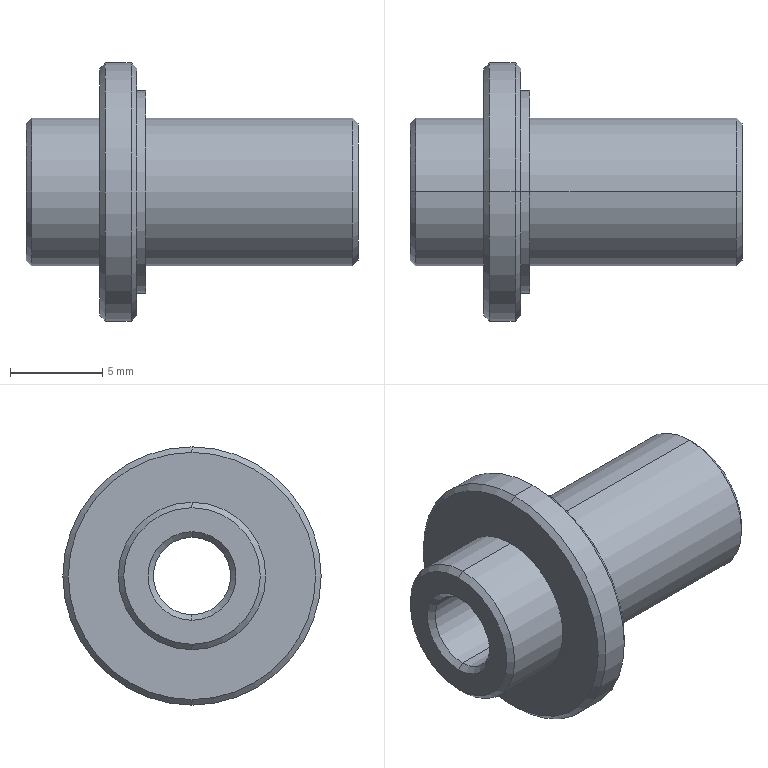Part | NX | features BREP 1 | 1 solid | 27 faces | box 18 x 14 x 14 mm | volume 877.777 mm3 | cone 12 | cylinder 10 | plane 5 | commonest cylinder face diameters 8 x4 4.2 x2 11 x2 14 x2
STEP:
#1=CARTESIAN_POINT('',(17.7,0.,2.1));
#2=VERTEX_POINT('',#1);
#3=CARTESIAN_POINT('',(17.7,0.,-2.1));
#4=VERTEX_POINT('',#3);
#5=CARTESIAN_POINT('',(17.7,0.,0.));
#6=DIRECTION('',(1.,0.,0.));
#7=DIRECTION('',(0.,0.,-1.));
#8=AXIS2_PLACEMENT_3D('',#5,#6,#7);
#9=CIRCLE('',#8,2.1);
#10=EDGE_CURVE('',#2,#4,#9,.T.);
#11=ORIENTED_EDGE('',*,*,#10,.F.);
#12=CARTESIAN_POINT('',(18.,0.,2.4));
#13=VERTEX_POINT('',#12);
#14=CARTESIAN_POINT('',(18.,0.,2.4));
#15=DIRECTION('',(0.7071,0.,0.7071));
#16=VECTOR('',#15,1000.);
#17=LINE('',#14,#16);
#18=EDGE_CURVE('',#2,#13,#17,.T.);
#19=ORIENTED_EDGE('',*,*,#18,.T.);
#20=CARTESIAN_POINT('',(18.,0.,-2.4));
#21=VERTEX_POINT('',#20);
#22=CARTESIAN_POINT('',(18.,0.,0.));
#23=DIRECTION('',(-1.,0.,0.));
#24=DIRECTION('',(0.,0.,-1.));
#25=AXIS2_PLACEMENT_3D('',#22,#23,#24);
#26=CIRCLE('',#25,2.4);
#27=EDGE_CURVE('',#21,#13,#26,.T.);
#28=ORIENTED_EDGE('',*,*,#27,.F.);
#29=CARTESIAN_POINT('',(18.,0.,-2.4));
#30=DIRECTION('',(0.7071,0.,-0.7071));
#31=VECTOR('',#30,1000.);
#32=LINE('',#29,#31);
#33=EDGE_CURVE('',#4,#21,#32,.T.);
#34=ORIENTED_EDGE('',*,*,#33,.F.);
#35=EDGE_LOOP('',(#11,#19,#28,#34));
#36=FACE_BOUND('',#35,.T.);
#37=CARTESIAN_POINT('',(18.,0.,0.));
#38=DIRECTION('',(1.,0.,0.));
#39=DIRECTION('',(0.,0.,-1.));
#40=AXIS2_PLACEMENT_3D('',#37,#38,#39);
#41=CONICAL_SURFACE('',#40,2.4,0.7854);
#42=ADVANCED_FACE('',(#36),#41,.F.);
#43=CARTESIAN_POINT('',(18.,0.,-3.7));
#44=VERTEX_POINT('',#43);
#45=CARTESIAN_POINT('',(18.,0.,3.7));
#46=VERTEX_POINT('',#45);
#47=CARTESIAN_POINT('',(18.,0.,0.));
#48=DIRECTION('',(1.,0.,0.));
#49=DIRECTION('',(0.,0.,-1.));
#50=AXIS2_PLACEMENT_3D('',#47,#48,#49);
#51=CIRCLE('',#50,3.7);
#52=EDGE_CURVE('',#44,#46,#51,.T.);
#53=ORIENTED_EDGE('',*,*,#52,.F.);
#54=CARTESIAN_POINT('',(17.7,0.,-4.));
#55=VERTEX_POINT('',#54);
#56=CARTESIAN_POINT('',(18.,0.,-3.7));
#57=DIRECTION('',(-0.7071,0.,-0.7071));
#58=VECTOR('',#57,1000.);
#59=LINE('',#56,#58);
#60=EDGE_CURVE('',#55,#44,#59,.F.);
#61=ORIENTED_EDGE('',*,*,#60,.F.);
#62=CARTESIAN_POINT('',(17.7,0.,4.));
#63=VERTEX_POINT('',#62);
#64=CARTESIAN_POINT('',(17.7,0.,0.));
#65=DIRECTION('',(-1.,0.,0.));
#66=DIRECTION('',(0.,0.,-1.));
#67=AXIS2_PLACEMENT_3D('',#64,#65,#66);
#68=CIRCLE('',#67,4.);
#69=EDGE_CURVE('',#63,#55,#68,.T.);
#70=ORIENTED_EDGE('',*,*,#69,.F.);
#71=CARTESIAN_POINT('',(18.,0.,3.7));
#72=DIRECTION('',(-0.7071,0.,0.7071));
#73=VECTOR('',#72,1000.);
#74=LINE('',#71,#73);
#75=EDGE_CURVE('',#63,#46,#74,.F.);
#76=ORIENTED_EDGE('',*,*,#75,.T.);
#77=EDGE_LOOP('',(#53,#61,#70,#76));
#78=FACE_BOUND('',#77,.T.);
#79=CARTESIAN_POINT('',(18.,0.,0.));
#80=DIRECTION('',(-1.,0.,0.));
#81=DIRECTION('',(0.,0.,1.));
#82=AXIS2_PLACEMENT_3D('',#79,#80,#81);
#83=CONICAL_SURFACE('',#82,3.7,0.7854);
#84=ADVANCED_FACE('',(#78),#83,.T.);
#85=CARTESIAN_POINT('',(0.,0.,3.7));
#86=VERTEX_POINT('',#85);
#87=CARTESIAN_POINT('',(0.,0.,-3.7));
#88=VERTEX_POINT('',#87);
#89=CARTESIAN_POINT('',(0.,0.,0.));
#90=DIRECTION('',(-1.,0.,0.));
#91=DIRECTION('',(0.,0.,-1.));
#92=AXIS2_PLACEMENT_3D('',#89,#90,#91);
#93=CIRCLE('',#92,3.7);
#94=EDGE_CURVE('',#86,#88,#93,.T.);
#95=ORIENTED_EDGE('',*,*,#94,.F.);
#96=CARTESIAN_POINT('',(0.3,0.,4.));
#97=VERTEX_POINT('',#96);
#98=CARTESIAN_POINT('',(0.,0.,3.7));
#99=DIRECTION('',(0.7071,0.,0.7071));
#100=VECTOR('',#99,1000.);
#101=LINE('',#98,#100);
#102=EDGE_CURVE('',#86,#97,#101,.T.);
#103=ORIENTED_EDGE('',*,*,#102,.T.);
#104=CARTESIAN_POINT('',(0.3,0.,-4.));
#105=VERTEX_POINT('',#104);
#106=CARTESIAN_POINT('',(0.3,0.,0.));
#107=DIRECTION('',(1.,0.,0.));
#108=DIRECTION('',(0.,0.,-1.));
#109=AXIS2_PLACEMENT_3D('',#106,#107,#108);
#110=CIRCLE('',#109,4.);
#111=EDGE_CURVE('',#105,#97,#110,.T.);
#112=ORIENTED_EDGE('',*,*,#111,.F.);
#113=CARTESIAN_POINT('',(0.,0.,-3.7));
#114=DIRECTION('',(0.7071,0.,-0.7071));
#115=VECTOR('',#114,1000.);
#116=LINE('',#113,#115);
#117=EDGE_CURVE('',#88,#105,#116,.T.);
#118=ORIENTED_EDGE('',*,*,#117,.F.);
#119=EDGE_LOOP('',(#95,#103,#112,#118));
#120=FACE_BOUND('',#119,.T.);
#121=CARTESIAN_POINT('',(0.,0.,0.));
#122=DIRECTION('',(1.,0.,0.));
#123=DIRECTION('',(0.,0.,-1.));
#124=AXIS2_PLACEMENT_3D('',#121,#122,#123);
#125=CONICAL_SURFACE('',#124,3.7,0.7854);
#126=ADVANCED_FACE('',(#120),#125,.T.);
#127=CARTESIAN_POINT('',(0.3,0.,-2.1));
#128=VERTEX_POINT('',#127);
#129=CARTESIAN_POINT('',(0.3,0.,2.1));
#130=VERTEX_POINT('',#129);
#131=CARTESIAN_POINT('',(0.3,0.,0.));
#132=DIRECTION('',(-1.,0.,0.));
#133=DIRECTION('',(0.,0.,-1.));
#134=AXIS2_PLACEMENT_3D('',#131,#132,#133);
#135=CIRCLE('',#134,2.1);
#136=EDGE_CURVE('',#128,#130,#135,.T.);
#137=ORIENTED_EDGE('',*,*,#136,.F.);
#138=CARTESIAN_POINT('',(0.,0.,-2.4));
#139=VERTEX_POINT('',#138);
#140=CARTESIAN_POINT('',(0.3,0.,-2.1));
#141=DIRECTION('',(-0.7071,0.,-0.7071));
#142=VECTOR('',#141,1000.);
#143=LINE('',#140,#142);
#144=EDGE_CURVE('',#139,#128,#143,.F.);
#145=ORIENTED_EDGE('',*,*,#144,.F.);
#146=CARTESIAN_POINT('',(0.,0.,2.4));
#147=VERTEX_POINT('',#146);
#148=CARTESIAN_POINT('',(0.,0.,0.));
#149=DIRECTION('',(1.,0.,0.));
#150=DIRECTION('',(0.,0.,-1.));
#151=AXIS2_PLACEMENT_3D('',#148,#149,#150);
#152=CIRCLE('',#151,2.4);
#153=EDGE_CURVE('',#147,#139,#152,.T.);
#154=ORIENTED_EDGE('',*,*,#153,.F.);
#155=CARTESIAN_POINT('',(0.3,0.,2.1));
#156=DIRECTION('',(-0.7071,0.,0.7071));
#157=VECTOR('',#156,1000.);
#158=LINE('',#155,#157);
#159=EDGE_CURVE('',#147,#130,#158,.F.);
#160=ORIENTED_EDGE('',*,*,#159,.T.);
#161=EDGE_LOOP('',(#137,#145,#154,#160));
#162=FACE_BOUND('',#161,.T.);
#163=CARTESIAN_POINT('',(0.3,0.,0.));
#164=DIRECTION('',(-1.,0.,0.));
#165=DIRECTION('',(0.,0.,1.));
#166=AXIS2_PLACEMENT_3D('',#163,#164,#165);
#167=CONICAL_SURFACE('',#166,2.1,0.7854);
#168=ADVANCED_FACE('',(#162),#167,.F.);
#169=CARTESIAN_POINT('',(4.,0.,6.7));
#170=VERTEX_POINT('',#169);
#171=CARTESIAN_POINT('',(4.,0.,-6.7));
#172=VERTEX_POINT('',#171);
#173=CARTESIAN_POINT('',(4.,0.,0.));
#174=DIRECTION('',(-1.,0.,0.));
#175=DIRECTION('',(0.,0.,-1.));
#176=AXIS2_PLACEMENT_3D('',#173,#174,#175);
#177=CIRCLE('',#176,6.7);
#178=EDGE_CURVE('',#170,#172,#177,.T.);
#179=ORIENTED_EDGE('',*,*,#178,.F.);
#180=CARTESIAN_POINT('',(4.3,0.,7.));
#181=VERTEX_POINT('',#180);
#182=CARTESIAN_POINT('',(4.,0.,6.7));
#183=DIRECTION('',(0.7071,0.,0.7071));
#184=VECTOR('',#183,1000.);
#185=LINE('',#182,#184);
#186=EDGE_CURVE('',#170,#181,#185,.T.);
#187=ORIENTED_EDGE('',*,*,#186,.T.);
#188=CARTESIAN_POINT('',(4.3,0.,-7.));
#189=VERTEX_POINT('',#188);
#190=CARTESIAN_POINT('',(4.3,0.,0.));
#191=DIRECTION('',(1.,0.,0.));
#192=DIRECTION('',(0.,0.,-1.));
#193=AXIS2_PLACEMENT_3D('',#190,#191,#192);
#194=CIRCLE('',#193,7.);
#195=EDGE_CURVE('',#189,#181,#194,.T.);
#196=ORIENTED_EDGE('',*,*,#195,.F.);
#197=CARTESIAN_POINT('',(4.,0.,-6.7));
#198=DIRECTION('',(0.7071,0.,-0.7071));
#199=VECTOR('',#198,1000.);
#200=LINE('',#197,#199);
#201=EDGE_CURVE('',#172,#189,#200,.T.);
#202=ORIENTED_EDGE('',*,*,#201,.F.);
#203=EDGE_LOOP('',(#179,#187,#196,#202));
#204=FACE_BOUND('',#203,.T.);
#205=CARTESIAN_POINT('',(4.,0.,0.));
#206=DIRECTION('',(1.,0.,0.));
#207=DIRECTION('',(0.,0.,-1.));
#208=AXIS2_PLACEMENT_3D('',#205,#206,#207);
#209=CONICAL_SURFACE('',#208,6.7,0.7854);
#210=ADVANCED_FACE('',(#204),#209,.T.);
#211=CARTESIAN_POINT('',(6.,0.,-6.7));
#212=VERTEX_POINT('',#211);
#213=CARTESIAN_POINT('',(6.,0.,6.7));
#214=VERTEX_POINT('',#213);
#215=CARTESIAN_POINT('',(6.,0.,0.));
#216=DIRECTION('',(1.,0.,0.));
#217=DIRECTION('',(0.,0.,1.));
#218=AXIS2_PLACEMENT_3D('',#215,#216,#217);
#219=CIRCLE('',#218,6.7);
#220=EDGE_CURVE('',#212,#214,#219,.T.);
#221=ORIENTED_EDGE('',*,*,#220,.F.);
#222=CARTESIAN_POINT('',(5.7,0.,-7.));
#223=VERTEX_POINT('',#222);
#224=CARTESIAN_POINT('',(5.7,0.,-7.));
#225=DIRECTION('',(-0.7071,0.,-0.7071));
#226=VECTOR('',#225,1000.);
#227=LINE('',#224,#226);
#228=EDGE_CURVE('',#223,#212,#227,.F.);
#229=ORIENTED_EDGE('',*,*,#228,.F.);
#230=CARTESIAN_POINT('',(5.7,0.,7.));
#231=VERTEX_POINT('',#230);
#232=CARTESIAN_POINT('',(5.7,0.,0.));
#233=DIRECTION('',(-1.,0.,0.));
#234=DIRECTION('',(0.,0.,1.));
#235=AXIS2_PLACEMENT_3D('',#232,#233,#234);
#236=CIRCLE('',#235,7.);
#237=EDGE_CURVE('',#231,#223,#236,.T.);
#238=ORIENTED_EDGE('',*,*,#237,.F.);
#239=CARTESIAN_POINT('',(5.7,0.,7.));
#240=DIRECTION('',(-0.7071,0.,0.7071));
#241=VECTOR('',#240,1000.);
#242=LINE('',#239,#241);
#243=EDGE_CURVE('',#231,#214,#242,.F.);
#244=ORIENTED_EDGE('',*,*,#243,.T.);
#245=EDGE_LOOP('',(#221,#229,#238,#244));
#246=FACE_BOUND('',#245,.T.);
#247=CARTESIAN_POINT('',(5.7,0.,0.));
#248=DIRECTION('',(-1.,0.,0.));
#249=DIRECTION('',(0.,0.,1.));
#250=AXIS2_PLACEMENT_3D('',#247,#248,#249);
#251=CONICAL_SURFACE('',#250,7.,0.7854);
#252=ADVANCED_FACE('',(#246),#251,.T.);
#253=ORIENTED_EDGE('',*,*,#237,.T.);
#254=CARTESIAN_POINT('',(0.,0.,-7.));
#255=DIRECTION('',(-1.,0.,0.));
#256=VECTOR('',#255,1000.);
#257=LINE('',#254,#256);
#258=EDGE_CURVE('',#189,#223,#257,.F.);
#259=ORIENTED_EDGE('',*,*,#258,.F.);
#260=ORIENTED_EDGE('',*,*,#195,.T.);
#261=CARTESIAN_POINT('',(0.,0.,7.));
#262=DIRECTION('',(-1.,0.,0.));
#263=VECTOR('',#262,1000.);
#264=LINE('',#261,#263);
#265=EDGE_CURVE('',#181,#231,#264,.F.);
#266=ORIENTED_EDGE('',*,*,#265,.T.);
#267=EDGE_LOOP('',(#253,#259,#260,#266));
#268=FACE_BOUND('',#267,.T.);
#269=CARTESIAN_POINT('',(0.,0.,0.));
#270=DIRECTION('',(-1.,0.,0.));
#271=DIRECTION('',(0.,0.,1.));
#272=AXIS2_PLACEMENT_3D('',#269,#270,#271);
#273=CYLINDRICAL_SURFACE('',#272,7.);
#274=ADVANCED_FACE('',(#268),#273,.T.);
#275=CARTESIAN_POINT('',(4.,0.,4.));
#276=VERTEX_POINT('',#275);
#277=CARTESIAN_POINT('',(4.,0.,-4.));
#278=VERTEX_POINT('',#277);
#279=CARTESIAN_POINT('',(4.,0.,0.));
#280=DIRECTION('',(-1.,0.,0.));
#281=DIRECTION('',(0.,0.,1.));
#282=AXIS2_PLACEMENT_3D('',#279,#280,#281);
#283=CIRCLE('',#282,4.);
#284=EDGE_CURVE('',#276,#278,#283,.T.);
#285=ORIENTED_EDGE('',*,*,#284,.T.);
#286=CARTESIAN_POINT('',(0.,0.,-4.));
#287=DIRECTION('',(-1.,0.,0.));
#288=VECTOR('',#287,1000.);
#289=LINE('',#286,#288);
#290=EDGE_CURVE('',#105,#278,#289,.F.);
#291=ORIENTED_EDGE('',*,*,#290,.F.);
#292=ORIENTED_EDGE('',*,*,#111,.T.);
#293=CARTESIAN_POINT('',(0.,0.,4.));
#294=DIRECTION('',(-1.,0.,0.));
#295=VECTOR('',#294,1000.);
#296=LINE('',#293,#295);
#297=EDGE_CURVE('',#97,#276,#296,.F.);
#298=ORIENTED_EDGE('',*,*,#297,.T.);
#299=EDGE_LOOP('',(#285,#291,#292,#298));
#300=FACE_BOUND('',#299,.T.);
#301=CARTESIAN_POINT('',(0.,0.,0.));
#302=DIRECTION('',(-1.,0.,0.));
#303=DIRECTION('',(0.,0.,1.));
#304=AXIS2_PLACEMENT_3D('',#301,#302,#303);
#305=CYLINDRICAL_SURFACE('',#304,4.);
#306=ADVANCED_FACE('',(#300),#305,.T.);
#307=CARTESIAN_POINT('',(6.5,0.,-5.5));
#308=VERTEX_POINT('',#307);
#309=CARTESIAN_POINT('',(6.5,0.,5.5));
#310=VERTEX_POINT('',#309);
#311=CARTESIAN_POINT('',(6.5,0.,0.));
#312=DIRECTION('',(1.,0.,0.));
#313=DIRECTION('',(0.,0.,-1.));
#314=AXIS2_PLACEMENT_3D('',#311,#312,#313);
#315=CIRCLE('',#314,5.5);
#316=EDGE_CURVE('',#308,#310,#315,.T.);
#317=ORIENTED_EDGE('',*,*,#316,.F.);
#318=CARTESIAN_POINT('',(6.,0.,-5.5));
#319=VERTEX_POINT('',#318);
#320=CARTESIAN_POINT('',(0.,0.,-5.5));
#321=DIRECTION('',(-1.,0.,0.));
#322=VECTOR('',#321,1000.);
#323=LINE('',#320,#322);
#324=EDGE_CURVE('',#319,#308,#323,.F.);
#325=ORIENTED_EDGE('',*,*,#324,.F.);
#326=CARTESIAN_POINT('',(6.,0.,5.5));
#327=VERTEX_POINT('',#326);
#328=CARTESIAN_POINT('',(6.,0.,0.));
#329=DIRECTION('',(-1.,0.,0.));
#330=DIRECTION('',(0.,0.,1.));
#331=AXIS2_PLACEMENT_3D('',#328,#329,#330);
#332=CIRCLE('',#331,5.5);
#333=EDGE_CURVE('',#327,#319,#332,.T.);
#334=ORIENTED_EDGE('',*,*,#333,.F.);
#335=CARTESIAN_POINT('',(0.,0.,5.5));
#336=DIRECTION('',(-1.,0.,0.));
#337=VECTOR('',#336,1000.);
#338=LINE('',#335,#337);
#339=EDGE_CURVE('',#327,#310,#338,.F.);
#340=ORIENTED_EDGE('',*,*,#339,.T.);
#341=EDGE_LOOP('',(#317,#325,#334,#340));
#342=FACE_BOUND('',#341,.T.);
#343=CARTESIAN_POINT('',(0.,0.,0.));
#344=DIRECTION('',(-1.,0.,0.));
#345=DIRECTION('',(0.,0.,1.));
#346=AXIS2_PLACEMENT_3D('',#343,#344,#345);
#347=CYLINDRICAL_SURFACE('',#346,5.5);
#348=ADVANCED_FACE('',(#342),#347,.T.);
#349=ORIENTED_EDGE('',*,*,#69,.T.);
#350=CARTESIAN_POINT('',(6.5,0.,-4.));
#351=VERTEX_POINT('',#350);
#352=CARTESIAN_POINT('',(0.,0.,-4.));
#353=DIRECTION('',(-1.,0.,0.));
#354=VECTOR('',#353,1000.);
#355=LINE('',#352,#354);
#356=EDGE_CURVE('',#351,#55,#355,.F.);
#357=ORIENTED_EDGE('',*,*,#356,.F.);
#358=CARTESIAN_POINT('',(6.5,0.,4.));
#359=VERTEX_POINT('',#358);
#360=CARTESIAN_POINT('',(6.5,0.,0.));
#361=DIRECTION('',(1.,0.,0.));
#362=DIRECTION('',(0.,0.,-1.));
#363=AXIS2_PLACEMENT_3D('',#360,#361,#362);
#364=CIRCLE('',#363,4.);
#365=EDGE_CURVE('',#351,#359,#364,.T.);
#366=ORIENTED_EDGE('',*,*,#365,.T.);
#367=CARTESIAN_POINT('',(0.,0.,4.));
#368=DIRECTION('',(-1.,0.,0.));
#369=VECTOR('',#368,1000.);
#370=LINE('',#367,#369);
#371=EDGE_CURVE('',#359,#63,#370,.F.);
#372=ORIENTED_EDGE('',*,*,#371,.T.);
#373=EDGE_LOOP('',(#349,#357,#366,#372));
#374=FACE_BOUND('',#373,.T.);
#375=CARTESIAN_POINT('',(0.,0.,0.));
#376=DIRECTION('',(-1.,0.,0.));
#377=DIRECTION('',(0.,0.,1.));
#378=AXIS2_PLACEMENT_3D('',#375,#376,#377);
#379=CYLINDRICAL_SURFACE('',#378,4.);
#380=ADVANCED_FACE('',(#374),#379,.T.);
#381=ORIENTED_EDGE('',*,*,#10,.T.);
#382=CARTESIAN_POINT('',(0.,0.,-2.1));
#383=DIRECTION('',(-1.,0.,0.));
#384=VECTOR('',#383,1000.);
#385=LINE('',#382,#384);
#386=EDGE_CURVE('',#128,#4,#385,.F.);
#387=ORIENTED_EDGE('',*,*,#386,.F.);
#388=ORIENTED_EDGE('',*,*,#136,.T.);
#389=CARTESIAN_POINT('',(0.,0.,2.1));
#390=DIRECTION('',(-1.,0.,0.));
#391=VECTOR('',#390,1000.);
#392=LINE('',#389,#391);
#393=EDGE_CURVE('',#130,#2,#392,.F.);
#394=ORIENTED_EDGE('',*,*,#393,.T.);
#395=EDGE_LOOP('',(#381,#387,#388,#394));
#396=FACE_BOUND('',#395,.T.);
#397=CARTESIAN_POINT('',(0.,0.,0.));
#398=DIRECTION('',(-1.,0.,0.));
#399=DIRECTION('',(0.,0.,1.));
#400=AXIS2_PLACEMENT_3D('',#397,#398,#399);
#401=CYLINDRICAL_SURFACE('',#400,2.1);
#402=ADVANCED_FACE('',(#396),#401,.F.);
#403=ORIENTED_EDGE('',*,*,#386,.T.);
#404=CARTESIAN_POINT('',(17.7,0.,0.));
#405=DIRECTION('',(1.,0.,0.));
#406=DIRECTION('',(0.,0.,-1.));
#407=AXIS2_PLACEMENT_3D('',#404,#405,#406);
#408=CIRCLE('',#407,2.1);
#409=EDGE_CURVE('',#4,#2,#408,.T.);
#410=ORIENTED_EDGE('',*,*,#409,.T.);
#411=ORIENTED_EDGE('',*,*,#393,.F.);
#412=CARTESIAN_POINT('',(0.3,0.,0.));
#413=DIRECTION('',(-1.,0.,0.));
#414=DIRECTION('',(0.,0.,-1.));
#415=AXIS2_PLACEMENT_3D('',#412,#413,#414);
#416=CIRCLE('',#415,2.1);
#417=EDGE_CURVE('',#130,#128,#416,.T.);
#418=ORIENTED_EDGE('',*,*,#417,.T.);
#419=EDGE_LOOP('',(#403,#410,#411,#418));
#420=FACE_BOUND('',#419,.T.);
#421=CARTESIAN_POINT('',(0.,0.,0.));
#422=DIRECTION('',(-1.,0.,0.));
#423=DIRECTION('',(0.,0.,1.));
#424=AXIS2_PLACEMENT_3D('',#421,#422,#423);
#425=CYLINDRICAL_SURFACE('',#424,2.1);
#426=ADVANCED_FACE('',(#420),#425,.F.);
#427=ORIENTED_EDGE('',*,*,#356,.T.);
#428=CARTESIAN_POINT('',(17.7,0.,0.));
#429=DIRECTION('',(-1.,0.,0.));
#430=DIRECTION('',(0.,0.,-1.));
#431=AXIS2_PLACEMENT_3D('',#428,#429,#430);
#432=CIRCLE('',#431,4.);
#433=EDGE_CURVE('',#55,#63,#432,.T.);
#434=ORIENTED_EDGE('',*,*,#433,.T.);
#435=ORIENTED_EDGE('',*,*,#371,.F.);
#436=CARTESIAN_POINT('',(6.5,0.,0.));
#437=DIRECTION('',(1.,0.,0.));
#438=DIRECTION('',(0.,0.,-1.));
#439=AXIS2_PLACEMENT_3D('',#436,#437,#438);
#440=CIRCLE('',#439,4.);
#441=EDGE_CURVE('',#359,#351,#440,.T.);
#442=ORIENTED_EDGE('',*,*,#441,.T.);
#443=EDGE_LOOP('',(#427,#434,#435,#442));
#444=FACE_BOUND('',#443,.T.);
#445=CARTESIAN_POINT('',(0.,0.,0.));
#446=DIRECTION('',(-1.,0.,0.));
#447=DIRECTION('',(0.,0.,1.));
#448=AXIS2_PLACEMENT_3D('',#445,#446,#447);
#449=CYLINDRICAL_SURFACE('',#448,4.);
#450=ADVANCED_FACE('',(#444),#449,.T.);
#451=ORIENTED_EDGE('',*,*,#324,.T.);
#452=CARTESIAN_POINT('',(6.5,0.,0.));
#453=DIRECTION('',(1.,0.,0.));
#454=DIRECTION('',(0.,0.,-1.));
#455=AXIS2_PLACEMENT_3D('',#452,#453,#454);
#456=CIRCLE('',#455,5.5);
#457=EDGE_CURVE('',#310,#308,#456,.T.);
#458=ORIENTED_EDGE('',*,*,#457,.F.);
#459=ORIENTED_EDGE('',*,*,#339,.F.);
#460=CARTESIAN_POINT('',(6.,0.,0.));
#461=DIRECTION('',(-1.,0.,0.));
#462=DIRECTION('',(0.,0.,1.));
#463=AXIS2_PLACEMENT_3D('',#460,#461,#462);
#464=CIRCLE('',#463,5.5);
#465=EDGE_CURVE('',#319,#327,#464,.T.);
#466=ORIENTED_EDGE('',*,*,#465,.F.);
#467=EDGE_LOOP('',(#451,#458,#459,#466));
#468=FACE_BOUND('',#467,.T.);
#469=CARTESIAN_POINT('',(0.,0.,0.));
#470=DIRECTION('',(-1.,0.,0.));
#471=DIRECTION('',(0.,0.,1.));
#472=AXIS2_PLACEMENT_3D('',#469,#470,#471);
#473=CYLINDRICAL_SURFACE('',#472,5.5);
#474=ADVANCED_FACE('',(#468),#473,.T.);
#475=CARTESIAN_POINT('',(0.,0.,0.));
#476=DIRECTION('',(-1.,0.,0.));
#477=DIRECTION('',(0.,0.,-1.));
#478=AXIS2_PLACEMENT_3D('',#475,#476,#477);
#479=CIRCLE('',#478,3.7);
#480=EDGE_CURVE('',#88,#86,#479,.T.);
#481=ORIENTED_EDGE('',*,*,#480,.T.);
#482=ORIENTED_EDGE('',*,*,#94,.T.);
#483=EDGE_LOOP('',(#481,#482));
#484=FACE_BOUND('',#483,.T.);
#485=ORIENTED_EDGE('',*,*,#153,.T.);
#486=CARTESIAN_POINT('',(0.,0.,0.));
#487=DIRECTION('',(1.,0.,0.));
#488=DIRECTION('',(0.,0.,-1.));
#489=AXIS2_PLACEMENT_3D('',#486,#487,#488);
#490=CIRCLE('',#489,2.4);
#491=EDGE_CURVE('',#139,#147,#490,.T.);
#492=ORIENTED_EDGE('',*,*,#491,.T.);
#493=EDGE_LOOP('',(#485,#492));
#494=FACE_BOUND('',#493,.T.);
#495=CARTESIAN_POINT('',(0.,2.1,0.));
#496=DIRECTION('',(1.,0.,0.));
#497=DIRECTION('',(0.,1.,0.));
#498=AXIS2_PLACEMENT_3D('',#495,#496,#497);
#499=PLANE('',#498);
#500=ADVANCED_FACE('',(#484,#494),#499,.F.);
#501=ORIENTED_EDGE('',*,*,#290,.T.);
#502=CARTESIAN_POINT('',(4.,0.,0.));
#503=DIRECTION('',(-1.,0.,0.));
#504=DIRECTION('',(0.,0.,1.));
#505=AXIS2_PLACEMENT_3D('',#502,#503,#504);
#506=CIRCLE('',#505,4.);
#507=EDGE_CURVE('',#278,#276,#506,.T.);
#508=ORIENTED_EDGE('',*,*,#507,.T.);
#509=ORIENTED_EDGE('',*,*,#297,.F.);
#510=CARTESIAN_POINT('',(0.3,0.,0.));
#511=DIRECTION('',(1.,0.,0.));
#512=DIRECTION('',(0.,0.,-1.));
#513=AXIS2_PLACEMENT_3D('',#510,#511,#512);
#514=CIRCLE('',#513,4.);
#515=EDGE_CURVE('',#97,#105,#514,.T.);
#516=ORIENTED_EDGE('',*,*,#515,.T.);
#517=EDGE_LOOP('',(#501,#508,#509,#516));
#518=FACE_BOUND('',#517,.T.);
#519=CARTESIAN_POINT('',(0.,0.,0.));
#520=DIRECTION('',(-1.,0.,0.));
#521=DIRECTION('',(0.,0.,1.));
#522=AXIS2_PLACEMENT_3D('',#519,#520,#521);
#523=CYLINDRICAL_SURFACE('',#522,4.);
#524=ADVANCED_FACE('',(#518),#523,.T.);
#525=CARTESIAN_POINT('',(4.,0.,0.));
#526=DIRECTION('',(-1.,0.,0.));
#527=DIRECTION('',(0.,0.,-1.));
#528=AXIS2_PLACEMENT_3D('',#525,#526,#527);
#529=CIRCLE('',#528,6.7);
#530=EDGE_CURVE('',#172,#170,#529,.T.);
#531=ORIENTED_EDGE('',*,*,#530,.T.);
#532=ORIENTED_EDGE('',*,*,#178,.T.);
#533=EDGE_LOOP('',(#531,#532));
#534=FACE_BOUND('',#533,.T.);
#535=ORIENTED_EDGE('',*,*,#284,.F.);
#536=ORIENTED_EDGE('',*,*,#507,.F.);
#537=EDGE_LOOP('',(#535,#536));
#538=FACE_BOUND('',#537,.T.);
#539=CARTESIAN_POINT('',(4.,4.,0.));
#540=DIRECTION('',(1.,0.,0.));
#541=DIRECTION('',(0.,1.,0.));
#542=AXIS2_PLACEMENT_3D('',#539,#540,#541);
#543=PLANE('',#542);
#544=ADVANCED_FACE('',(#534,#538),#543,.F.);
#545=ORIENTED_EDGE('',*,*,#258,.T.);
#546=CARTESIAN_POINT('',(5.7,0.,0.));
#547=DIRECTION('',(-1.,0.,0.));
#548=DIRECTION('',(0.,0.,1.));
#549=AXIS2_PLACEMENT_3D('',#546,#547,#548);
#550=CIRCLE('',#549,7.);
#551=EDGE_CURVE('',#223,#231,#550,.T.);
#552=ORIENTED_EDGE('',*,*,#551,.T.);
#553=ORIENTED_EDGE('',*,*,#265,.F.);
#554=CARTESIAN_POINT('',(4.3,0.,0.));
#555=DIRECTION('',(1.,0.,0.));
#556=DIRECTION('',(0.,0.,-1.));
#557=AXIS2_PLACEMENT_3D('',#554,#555,#556);
#558=CIRCLE('',#557,7.);
#559=EDGE_CURVE('',#181,#189,#558,.T.);
#560=ORIENTED_EDGE('',*,*,#559,.T.);
#561=EDGE_LOOP('',(#545,#552,#553,#560));
#562=FACE_BOUND('',#561,.T.);
#563=CARTESIAN_POINT('',(0.,0.,0.));
#564=DIRECTION('',(-1.,0.,0.));
#565=DIRECTION('',(0.,0.,1.));
#566=AXIS2_PLACEMENT_3D('',#563,#564,#565);
#567=CYLINDRICAL_SURFACE('',#566,7.);
#568=ADVANCED_FACE('',(#562),#567,.T.);
#569=CARTESIAN_POINT('',(6.,0.,0.));
#570=DIRECTION('',(1.,0.,0.));
#571=DIRECTION('',(0.,0.,1.));
#572=AXIS2_PLACEMENT_3D('',#569,#570,#571);
#573=CIRCLE('',#572,6.7);
#574=EDGE_CURVE('',#214,#212,#573,.T.);
#575=ORIENTED_EDGE('',*,*,#574,.T.);
#576=ORIENTED_EDGE('',*,*,#220,.T.);
#577=EDGE_LOOP('',(#575,#576));
#578=FACE_BOUND('',#577,.T.);
#579=ORIENTED_EDGE('',*,*,#333,.T.);
#580=ORIENTED_EDGE('',*,*,#465,.T.);
#581=EDGE_LOOP('',(#579,#580));
#582=FACE_BOUND('',#581,.T.);
#583=CARTESIAN_POINT('',(6.,7.,0.));
#584=DIRECTION('',(-1.,0.,0.));
#585=DIRECTION('',(0.,0.,1.));
#586=AXIS2_PLACEMENT_3D('',#583,#584,#585);
#587=PLANE('',#586);
#588=ADVANCED_FACE('',(#578,#582),#587,.F.);
#589=ORIENTED_EDGE('',*,*,#228,.T.);
#590=ORIENTED_EDGE('',*,*,#574,.F.);
#591=ORIENTED_EDGE('',*,*,#243,.F.);
#592=ORIENTED_EDGE('',*,*,#551,.F.);
#593=EDGE_LOOP('',(#589,#590,#591,#592));
#594=FACE_BOUND('',#593,.T.);
#595=CARTESIAN_POINT('',(5.7,0.,0.));
#596=DIRECTION('',(-1.,0.,0.));
#597=DIRECTION('',(0.,0.,1.));
#598=AXIS2_PLACEMENT_3D('',#595,#596,#597);
#599=CONICAL_SURFACE('',#598,7.,0.7854);
#600=ADVANCED_FACE('',(#594),#599,.T.);
#601=ORIENTED_EDGE('',*,*,#186,.F.);
#602=ORIENTED_EDGE('',*,*,#530,.F.);
#603=ORIENTED_EDGE('',*,*,#201,.T.);
#604=ORIENTED_EDGE('',*,*,#559,.F.);
#605=EDGE_LOOP('',(#601,#602,#603,#604));
#606=FACE_BOUND('',#605,.T.);
#607=CARTESIAN_POINT('',(4.,0.,0.));
#608=DIRECTION('',(1.,0.,0.));
#609=DIRECTION('',(0.,0.,-1.));
#610=AXIS2_PLACEMENT_3D('',#607,#608,#609);
#611=CONICAL_SURFACE('',#610,6.7,0.7854);
#612=ADVANCED_FACE('',(#606),#611,.T.);
#613=ORIENTED_EDGE('',*,*,#144,.T.);
#614=ORIENTED_EDGE('',*,*,#417,.F.);
#615=ORIENTED_EDGE('',*,*,#159,.F.);
#616=ORIENTED_EDGE('',*,*,#491,.F.);
#617=EDGE_LOOP('',(#613,#614,#615,#616));
#618=FACE_BOUND('',#617,.T.);
#619=CARTESIAN_POINT('',(0.3,0.,0.));
#620=DIRECTION('',(-1.,0.,0.));
#621=DIRECTION('',(0.,0.,1.));
#622=AXIS2_PLACEMENT_3D('',#619,#620,#621);
#623=CONICAL_SURFACE('',#622,2.1,0.7854);
#624=ADVANCED_FACE('',(#618),#623,.F.);
#625=ORIENTED_EDGE('',*,*,#102,.F.);
#626=ORIENTED_EDGE('',*,*,#480,.F.);
#627=ORIENTED_EDGE('',*,*,#117,.T.);
#628=ORIENTED_EDGE('',*,*,#515,.F.);
#629=EDGE_LOOP('',(#625,#626,#627,#628));
#630=FACE_BOUND('',#629,.T.);
#631=CARTESIAN_POINT('',(0.,0.,0.));
#632=DIRECTION('',(1.,0.,0.));
#633=DIRECTION('',(0.,0.,-1.));
#634=AXIS2_PLACEMENT_3D('',#631,#632,#633);
#635=CONICAL_SURFACE('',#634,3.7,0.7854);
#636=ADVANCED_FACE('',(#630),#635,.T.);
#637=ORIENTED_EDGE('',*,*,#457,.T.);
#638=ORIENTED_EDGE('',*,*,#316,.T.);
#639=EDGE_LOOP('',(#637,#638));
#640=FACE_BOUND('',#639,.T.);
#641=ORIENTED_EDGE('',*,*,#441,.F.);
#642=ORIENTED_EDGE('',*,*,#365,.F.);
#643=EDGE_LOOP('',(#641,#642));
#644=FACE_BOUND('',#643,.T.);
#645=CARTESIAN_POINT('',(6.5,0.,0.));
#646=DIRECTION('',(1.,0.,0.));
#647=DIRECTION('',(0.,1.,0.));
#648=AXIS2_PLACEMENT_3D('',#645,#646,#647);
#649=PLANE('',#648);
#650=ADVANCED_FACE('',(#640,#644),#649,.T.);
#651=CARTESIAN_POINT('',(18.,0.,0.));
#652=DIRECTION('',(1.,0.,0.));
#653=DIRECTION('',(0.,0.,-1.));
#654=AXIS2_PLACEMENT_3D('',#651,#652,#653);
#655=CIRCLE('',#654,3.7);
#656=EDGE_CURVE('',#46,#44,#655,.T.);
#657=ORIENTED_EDGE('',*,*,#656,.T.);
#658=ORIENTED_EDGE('',*,*,#52,.T.);
#659=EDGE_LOOP('',(#657,#658));
#660=FACE_BOUND('',#659,.T.);
#661=ORIENTED_EDGE('',*,*,#27,.T.);
#662=CARTESIAN_POINT('',(18.,0.,0.));
#663=DIRECTION('',(-1.,0.,0.));
#664=DIRECTION('',(0.,0.,-1.));
#665=AXIS2_PLACEMENT_3D('',#662,#663,#664);
#666=CIRCLE('',#665,2.4);
#667=EDGE_CURVE('',#13,#21,#666,.T.);
#668=ORIENTED_EDGE('',*,*,#667,.T.);
#669=EDGE_LOOP('',(#661,#668));
#670=FACE_BOUND('',#669,.T.);
#671=CARTESIAN_POINT('',(18.,0.,0.));
#672=DIRECTION('',(1.,0.,0.));
#673=DIRECTION('',(0.,1.,0.));
#674=AXIS2_PLACEMENT_3D('',#671,#672,#673);
#675=PLANE('',#674);
#676=ADVANCED_FACE('',(#660,#670),#675,.T.);
#677=ORIENTED_EDGE('',*,*,#60,.T.);
#678=ORIENTED_EDGE('',*,*,#656,.F.);
#679=ORIENTED_EDGE('',*,*,#75,.F.);
#680=ORIENTED_EDGE('',*,*,#433,.F.);
#681=EDGE_LOOP('',(#677,#678,#679,#680));
#682=FACE_BOUND('',#681,.T.);
#683=CARTESIAN_POINT('',(18.,0.,0.));
#684=DIRECTION('',(-1.,0.,0.));
#685=DIRECTION('',(0.,0.,1.));
#686=AXIS2_PLACEMENT_3D('',#683,#684,#685);
#687=CONICAL_SURFACE('',#686,3.7,0.7854);
#688=ADVANCED_FACE('',(#682),#687,.T.);
#689=ORIENTED_EDGE('',*,*,#18,.F.);
#690=ORIENTED_EDGE('',*,*,#409,.F.);
#691=ORIENTED_EDGE('',*,*,#33,.T.);
#692=ORIENTED_EDGE('',*,*,#667,.F.);
#693=EDGE_LOOP('',(#689,#690,#691,#692));
#694=FACE_BOUND('',#693,.T.);
#695=CARTESIAN_POINT('',(18.,0.,0.));
#696=DIRECTION('',(1.,0.,0.));
#697=DIRECTION('',(0.,0.,-1.));
#698=AXIS2_PLACEMENT_3D('',#695,#696,#697);
#699=CONICAL_SURFACE('',#698,2.4,0.7854);
#700=ADVANCED_FACE('',(#694),#699,.F.);
#701=CLOSED_SHELL('',(#42,#84,#126,#168,#210,#252,#274,#306,#348,#380,#402,#426,#450,#474,#500,#524,#544,#568,#588,#600,#612,#624,#636,#650,#676,#688,#700));
#702=MANIFOLD_SOLID_BREP('',#701);
#703=(LENGTH_UNIT()NAMED_UNIT(*)SI_UNIT(.MILLI.,.METRE.));
#704=UNCERTAINTY_MEASURE_WITH_UNIT(LENGTH_MEASURE(0.00001),#703,'','');
#705=(NAMED_UNIT(*)PLANE_ANGLE_UNIT()SI_UNIT($,.RADIAN.));
#706=(NAMED_UNIT(*)SI_UNIT($,.STERADIAN.)SOLID_ANGLE_UNIT());
#707=(GEOMETRIC_REPRESENTATION_CONTEXT(3)GLOBAL_UNCERTAINTY_ASSIGNED_CONTEXT((#704))GLOBAL_UNIT_ASSIGNED_CONTEXT((#703,#705,#706))REPRESENTATION_CONTEXT('',''));
#708=ADVANCED_BREP_SHAPE_REPRESENTATION('',(#702),#707);